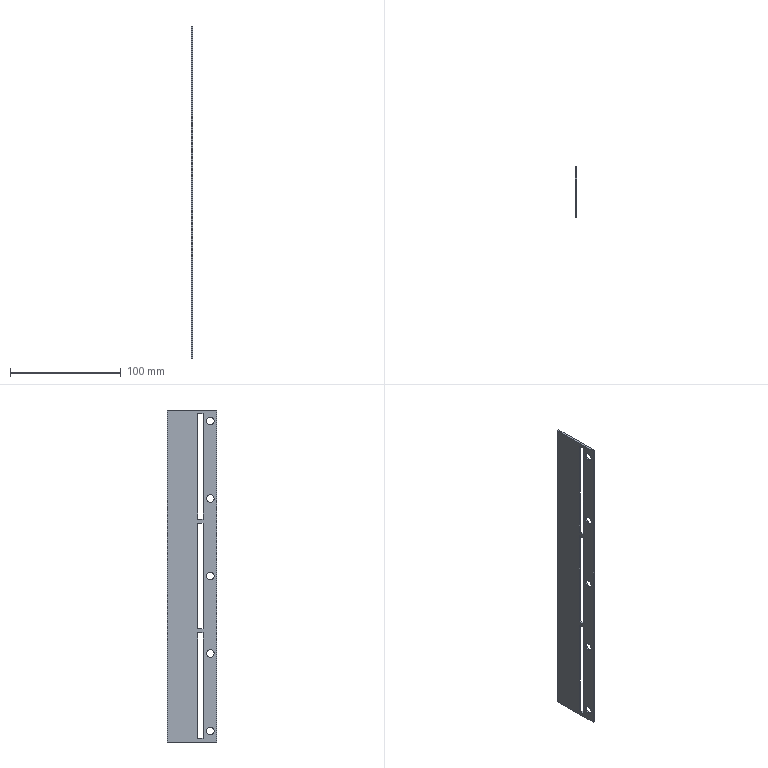Part | STEP file | SYL_0392D6J1SYL0380DJ10-1103933 | 1 solid | 28 faces | box 1.5 x 45 x 300 mm | volume 17824 mm3 | plane 18 | cylinder 10 | commonest cylinder face diameters 7 x10
STEP:
#1=CARTESIAN_POINT('',(0.,6.,-143.5));
#2=VERTEX_POINT('',#1);
#3=CARTESIAN_POINT('',(0.,6.,-136.5));
#4=VERTEX_POINT('',#3);
#5=CARTESIAN_POINT('',(0.,6.,-140.));
#6=DIRECTION('',(1.,0.,0.));
#7=DIRECTION('',(0.,0.,-1.));
#8=AXIS2_PLACEMENT_3D('',#5,#6,#7);
#9=CIRCLE('',#8,3.5);
#10=EDGE_CURVE('',#2,#4,#9,.T.);
#11=ORIENTED_EDGE('',*,*,#10,.F.);
#12=CARTESIAN_POINT('',(1.5,6.,-143.5));
#13=VERTEX_POINT('',#12);
#14=CARTESIAN_POINT('',(1.5,6.,-143.5));
#15=DIRECTION('',(-1.,0.,0.));
#16=VECTOR('',#15,1000.);
#17=LINE('',#14,#16);
#18=EDGE_CURVE('',#13,#2,#17,.T.);
#19=ORIENTED_EDGE('',*,*,#18,.F.);
#20=CARTESIAN_POINT('',(1.5,6.,-136.5));
#21=VERTEX_POINT('',#20);
#22=CARTESIAN_POINT('',(1.5,6.,-140.));
#23=DIRECTION('',(-1.,0.,0.));
#24=DIRECTION('',(0.,0.,1.));
#25=AXIS2_PLACEMENT_3D('',#22,#23,#24);
#26=CIRCLE('',#25,3.5);
#27=EDGE_CURVE('',#21,#13,#26,.T.);
#28=ORIENTED_EDGE('',*,*,#27,.F.);
#29=CARTESIAN_POINT('',(1.5,6.,-136.5));
#30=DIRECTION('',(-1.,0.,0.));
#31=VECTOR('',#30,1000.);
#32=LINE('',#29,#31);
#33=EDGE_CURVE('',#21,#4,#32,.T.);
#34=ORIENTED_EDGE('',*,*,#33,.T.);
#35=EDGE_LOOP('',(#11,#19,#28,#34));
#36=FACE_OUTER_BOUND('',#35,.T.);
#37=CARTESIAN_POINT('',(0.75,6.,-140.));
#38=DIRECTION('',(1.,0.,0.));
#39=DIRECTION('',(0.,0.,-1.));
#40=AXIS2_PLACEMENT_3D('',#37,#38,#39);
#41=CYLINDRICAL_SURFACE('',#40,3.5);
#42=ADVANCED_FACE('',(#36),#41,.F.);
#43=ORIENTED_EDGE('',*,*,#33,.F.);
#44=CARTESIAN_POINT('',(1.5,6.,-140.));
#45=DIRECTION('',(-1.,0.,0.));
#46=DIRECTION('',(0.,0.,-1.));
#47=AXIS2_PLACEMENT_3D('',#44,#45,#46);
#48=CIRCLE('',#47,3.5);
#49=EDGE_CURVE('',#13,#21,#48,.T.);
#50=ORIENTED_EDGE('',*,*,#49,.F.);
#51=ORIENTED_EDGE('',*,*,#18,.T.);
#52=CARTESIAN_POINT('',(0.,6.,-140.));
#53=DIRECTION('',(1.,0.,0.));
#54=DIRECTION('',(0.,0.,1.));
#55=AXIS2_PLACEMENT_3D('',#52,#53,#54);
#56=CIRCLE('',#55,3.5);
#57=EDGE_CURVE('',#4,#2,#56,.T.);
#58=ORIENTED_EDGE('',*,*,#57,.F.);
#59=EDGE_LOOP('',(#43,#50,#51,#58));
#60=FACE_OUTER_BOUND('',#59,.T.);
#61=CARTESIAN_POINT('',(0.75,6.,-140.));
#62=DIRECTION('',(1.,0.,0.));
#63=DIRECTION('',(0.,0.,-1.));
#64=AXIS2_PLACEMENT_3D('',#61,#62,#63);
#65=CYLINDRICAL_SURFACE('',#64,3.5);
#66=ADVANCED_FACE('',(#60),#65,.F.);
#67=CARTESIAN_POINT('',(0.,6.,136.5));
#68=VERTEX_POINT('',#67);
#69=CARTESIAN_POINT('',(0.,6.,143.5));
#70=VERTEX_POINT('',#69);
#71=CARTESIAN_POINT('',(0.,6.,140.));
#72=DIRECTION('',(1.,0.,0.));
#73=DIRECTION('',(0.,0.,-1.));
#74=AXIS2_PLACEMENT_3D('',#71,#72,#73);
#75=CIRCLE('',#74,3.5);
#76=EDGE_CURVE('',#68,#70,#75,.T.);
#77=ORIENTED_EDGE('',*,*,#76,.F.);
#78=CARTESIAN_POINT('',(1.5,6.,136.5));
#79=VERTEX_POINT('',#78);
#80=CARTESIAN_POINT('',(1.5,6.,136.5));
#81=DIRECTION('',(-1.,0.,0.));
#82=VECTOR('',#81,1000.);
#83=LINE('',#80,#82);
#84=EDGE_CURVE('',#79,#68,#83,.T.);
#85=ORIENTED_EDGE('',*,*,#84,.F.);
#86=CARTESIAN_POINT('',(1.5,6.,143.5));
#87=VERTEX_POINT('',#86);
#88=CARTESIAN_POINT('',(1.5,6.,140.));
#89=DIRECTION('',(-1.,0.,0.));
#90=DIRECTION('',(0.,0.,1.));
#91=AXIS2_PLACEMENT_3D('',#88,#89,#90);
#92=CIRCLE('',#91,3.5);
#93=EDGE_CURVE('',#87,#79,#92,.T.);
#94=ORIENTED_EDGE('',*,*,#93,.F.);
#95=CARTESIAN_POINT('',(1.5,6.,143.5));
#96=DIRECTION('',(-1.,0.,0.));
#97=VECTOR('',#96,1000.);
#98=LINE('',#95,#97);
#99=EDGE_CURVE('',#87,#70,#98,.T.);
#100=ORIENTED_EDGE('',*,*,#99,.T.);
#101=EDGE_LOOP('',(#77,#85,#94,#100));
#102=FACE_OUTER_BOUND('',#101,.T.);
#103=CARTESIAN_POINT('',(0.75,6.,140.));
#104=DIRECTION('',(1.,0.,0.));
#105=DIRECTION('',(0.,0.,-1.));
#106=AXIS2_PLACEMENT_3D('',#103,#104,#105);
#107=CYLINDRICAL_SURFACE('',#106,3.5);
#108=ADVANCED_FACE('',(#102),#107,.F.);
#109=ORIENTED_EDGE('',*,*,#99,.F.);
#110=CARTESIAN_POINT('',(1.5,6.,140.));
#111=DIRECTION('',(-1.,0.,0.));
#112=DIRECTION('',(0.,0.,-1.));
#113=AXIS2_PLACEMENT_3D('',#110,#111,#112);
#114=CIRCLE('',#113,3.5);
#115=EDGE_CURVE('',#79,#87,#114,.T.);
#116=ORIENTED_EDGE('',*,*,#115,.F.);
#117=ORIENTED_EDGE('',*,*,#84,.T.);
#118=CARTESIAN_POINT('',(0.,6.,140.));
#119=DIRECTION('',(1.,0.,0.));
#120=DIRECTION('',(0.,0.,1.));
#121=AXIS2_PLACEMENT_3D('',#118,#119,#120);
#122=CIRCLE('',#121,3.5);
#123=EDGE_CURVE('',#70,#68,#122,.T.);
#124=ORIENTED_EDGE('',*,*,#123,.F.);
#125=EDGE_LOOP('',(#109,#116,#117,#124));
#126=FACE_OUTER_BOUND('',#125,.T.);
#127=CARTESIAN_POINT('',(0.75,6.,140.));
#128=DIRECTION('',(1.,0.,0.));
#129=DIRECTION('',(0.,0.,-1.));
#130=AXIS2_PLACEMENT_3D('',#127,#128,#129);
#131=CYLINDRICAL_SURFACE('',#130,3.5);
#132=ADVANCED_FACE('',(#126),#131,.F.);
#133=CARTESIAN_POINT('',(0.,6.,-3.5));
#134=VERTEX_POINT('',#133);
#135=CARTESIAN_POINT('',(0.,6.,3.5));
#136=VERTEX_POINT('',#135);
#137=CARTESIAN_POINT('',(0.,6.,0.));
#138=DIRECTION('',(1.,0.,0.));
#139=DIRECTION('',(0.,0.,-1.));
#140=AXIS2_PLACEMENT_3D('',#137,#138,#139);
#141=CIRCLE('',#140,3.5);
#142=EDGE_CURVE('',#134,#136,#141,.T.);
#143=ORIENTED_EDGE('',*,*,#142,.F.);
#144=CARTESIAN_POINT('',(1.5,6.,-3.5));
#145=VERTEX_POINT('',#144);
#146=CARTESIAN_POINT('',(1.5,6.,-3.5));
#147=DIRECTION('',(-1.,0.,0.));
#148=VECTOR('',#147,1000.);
#149=LINE('',#146,#148);
#150=EDGE_CURVE('',#145,#134,#149,.T.);
#151=ORIENTED_EDGE('',*,*,#150,.F.);
#152=CARTESIAN_POINT('',(1.5,6.,3.5));
#153=VERTEX_POINT('',#152);
#154=CARTESIAN_POINT('',(1.5,6.,0.));
#155=DIRECTION('',(-1.,0.,0.));
#156=DIRECTION('',(0.,0.,1.));
#157=AXIS2_PLACEMENT_3D('',#154,#155,#156);
#158=CIRCLE('',#157,3.5);
#159=EDGE_CURVE('',#153,#145,#158,.T.);
#160=ORIENTED_EDGE('',*,*,#159,.F.);
#161=CARTESIAN_POINT('',(1.5,6.,3.5));
#162=DIRECTION('',(-1.,0.,0.));
#163=VECTOR('',#162,1000.);
#164=LINE('',#161,#163);
#165=EDGE_CURVE('',#153,#136,#164,.T.);
#166=ORIENTED_EDGE('',*,*,#165,.T.);
#167=EDGE_LOOP('',(#143,#151,#160,#166));
#168=FACE_OUTER_BOUND('',#167,.T.);
#169=CARTESIAN_POINT('',(0.75,6.,0.));
#170=DIRECTION('',(1.,0.,0.));
#171=DIRECTION('',(0.,0.,-1.));
#172=AXIS2_PLACEMENT_3D('',#169,#170,#171);
#173=CYLINDRICAL_SURFACE('',#172,3.5);
#174=ADVANCED_FACE('',(#168),#173,.F.);
#175=ORIENTED_EDGE('',*,*,#165,.F.);
#176=CARTESIAN_POINT('',(1.5,6.,0.));
#177=DIRECTION('',(-1.,0.,0.));
#178=DIRECTION('',(0.,0.,-1.));
#179=AXIS2_PLACEMENT_3D('',#176,#177,#178);
#180=CIRCLE('',#179,3.5);
#181=EDGE_CURVE('',#145,#153,#180,.T.);
#182=ORIENTED_EDGE('',*,*,#181,.F.);
#183=ORIENTED_EDGE('',*,*,#150,.T.);
#184=CARTESIAN_POINT('',(0.,6.,0.));
#185=DIRECTION('',(1.,0.,0.));
#186=DIRECTION('',(0.,0.,1.));
#187=AXIS2_PLACEMENT_3D('',#184,#185,#186);
#188=CIRCLE('',#187,3.5);
#189=EDGE_CURVE('',#136,#134,#188,.T.);
#190=ORIENTED_EDGE('',*,*,#189,.F.);
#191=EDGE_LOOP('',(#175,#182,#183,#190));
#192=FACE_OUTER_BOUND('',#191,.T.);
#193=CARTESIAN_POINT('',(0.75,6.,0.));
#194=DIRECTION('',(1.,0.,0.));
#195=DIRECTION('',(0.,0.,-1.));
#196=AXIS2_PLACEMENT_3D('',#193,#194,#195);
#197=CYLINDRICAL_SURFACE('',#196,3.5);
#198=ADVANCED_FACE('',(#192),#197,.F.);
#199=CARTESIAN_POINT('',(0.,6.,-73.5));
#200=VERTEX_POINT('',#199);
#201=CARTESIAN_POINT('',(0.,6.,-66.5));
#202=VERTEX_POINT('',#201);
#203=CARTESIAN_POINT('',(0.,6.,-70.));
#204=DIRECTION('',(1.,0.,0.));
#205=DIRECTION('',(0.,0.,-1.));
#206=AXIS2_PLACEMENT_3D('',#203,#204,#205);
#207=CIRCLE('',#206,3.5);
#208=EDGE_CURVE('',#200,#202,#207,.T.);
#209=ORIENTED_EDGE('',*,*,#208,.F.);
#210=CARTESIAN_POINT('',(1.5,6.,-73.5));
#211=VERTEX_POINT('',#210);
#212=CARTESIAN_POINT('',(1.5,6.,-73.5));
#213=DIRECTION('',(-1.,0.,0.));
#214=VECTOR('',#213,1000.);
#215=LINE('',#212,#214);
#216=EDGE_CURVE('',#211,#200,#215,.T.);
#217=ORIENTED_EDGE('',*,*,#216,.F.);
#218=CARTESIAN_POINT('',(1.5,6.,-66.5));
#219=VERTEX_POINT('',#218);
#220=CARTESIAN_POINT('',(1.5,6.,-70.));
#221=DIRECTION('',(-1.,0.,0.));
#222=DIRECTION('',(0.,0.,1.));
#223=AXIS2_PLACEMENT_3D('',#220,#221,#222);
#224=CIRCLE('',#223,3.5);
#225=EDGE_CURVE('',#219,#211,#224,.T.);
#226=ORIENTED_EDGE('',*,*,#225,.F.);
#227=CARTESIAN_POINT('',(1.5,6.,-66.5));
#228=DIRECTION('',(-1.,0.,0.));
#229=VECTOR('',#228,1000.);
#230=LINE('',#227,#229);
#231=EDGE_CURVE('',#219,#202,#230,.T.);
#232=ORIENTED_EDGE('',*,*,#231,.T.);
#233=EDGE_LOOP('',(#209,#217,#226,#232));
#234=FACE_OUTER_BOUND('',#233,.T.);
#235=CARTESIAN_POINT('',(0.75,6.,-70.));
#236=DIRECTION('',(1.,0.,0.));
#237=DIRECTION('',(0.,0.,-1.));
#238=AXIS2_PLACEMENT_3D('',#235,#236,#237);
#239=CYLINDRICAL_SURFACE('',#238,3.5);
#240=ADVANCED_FACE('',(#234),#239,.F.);
#241=ORIENTED_EDGE('',*,*,#231,.F.);
#242=CARTESIAN_POINT('',(1.5,6.,-70.));
#243=DIRECTION('',(-1.,0.,0.));
#244=DIRECTION('',(0.,0.,-1.));
#245=AXIS2_PLACEMENT_3D('',#242,#243,#244);
#246=CIRCLE('',#245,3.5);
#247=EDGE_CURVE('',#211,#219,#246,.T.);
#248=ORIENTED_EDGE('',*,*,#247,.F.);
#249=ORIENTED_EDGE('',*,*,#216,.T.);
#250=CARTESIAN_POINT('',(0.,6.,-70.));
#251=DIRECTION('',(1.,0.,0.));
#252=DIRECTION('',(0.,0.,1.));
#253=AXIS2_PLACEMENT_3D('',#250,#251,#252);
#254=CIRCLE('',#253,3.5);
#255=EDGE_CURVE('',#202,#200,#254,.T.);
#256=ORIENTED_EDGE('',*,*,#255,.F.);
#257=EDGE_LOOP('',(#241,#248,#249,#256));
#258=FACE_OUTER_BOUND('',#257,.T.);
#259=CARTESIAN_POINT('',(0.75,6.,-70.));
#260=DIRECTION('',(1.,0.,0.));
#261=DIRECTION('',(0.,0.,-1.));
#262=AXIS2_PLACEMENT_3D('',#259,#260,#261);
#263=CYLINDRICAL_SURFACE('',#262,3.5);
#264=ADVANCED_FACE('',(#258),#263,.F.);
#265=CARTESIAN_POINT('',(0.,6.,66.5));
#266=VERTEX_POINT('',#265);
#267=CARTESIAN_POINT('',(0.,6.,73.5));
#268=VERTEX_POINT('',#267);
#269=CARTESIAN_POINT('',(0.,6.,70.));
#270=DIRECTION('',(1.,0.,0.));
#271=DIRECTION('',(0.,0.,-1.));
#272=AXIS2_PLACEMENT_3D('',#269,#270,#271);
#273=CIRCLE('',#272,3.5);
#274=EDGE_CURVE('',#266,#268,#273,.T.);
#275=ORIENTED_EDGE('',*,*,#274,.F.);
#276=CARTESIAN_POINT('',(1.5,6.,66.5));
#277=VERTEX_POINT('',#276);
#278=CARTESIAN_POINT('',(1.5,6.,66.5));
#279=DIRECTION('',(-1.,0.,0.));
#280=VECTOR('',#279,1000.);
#281=LINE('',#278,#280);
#282=EDGE_CURVE('',#277,#266,#281,.T.);
#283=ORIENTED_EDGE('',*,*,#282,.F.);
#284=CARTESIAN_POINT('',(1.5,6.,73.5));
#285=VERTEX_POINT('',#284);
#286=CARTESIAN_POINT('',(1.5,6.,70.));
#287=DIRECTION('',(-1.,0.,0.));
#288=DIRECTION('',(0.,0.,1.));
#289=AXIS2_PLACEMENT_3D('',#286,#287,#288);
#290=CIRCLE('',#289,3.5);
#291=EDGE_CURVE('',#285,#277,#290,.T.);
#292=ORIENTED_EDGE('',*,*,#291,.F.);
#293=CARTESIAN_POINT('',(1.5,6.,73.5));
#294=DIRECTION('',(-1.,0.,0.));
#295=VECTOR('',#294,1000.);
#296=LINE('',#293,#295);
#297=EDGE_CURVE('',#285,#268,#296,.T.);
#298=ORIENTED_EDGE('',*,*,#297,.T.);
#299=EDGE_LOOP('',(#275,#283,#292,#298));
#300=FACE_OUTER_BOUND('',#299,.T.);
#301=CARTESIAN_POINT('',(0.75,6.,70.));
#302=DIRECTION('',(1.,0.,0.));
#303=DIRECTION('',(0.,0.,-1.));
#304=AXIS2_PLACEMENT_3D('',#301,#302,#303);
#305=CYLINDRICAL_SURFACE('',#304,3.5);
#306=ADVANCED_FACE('',(#300),#305,.F.);
#307=ORIENTED_EDGE('',*,*,#297,.F.);
#308=CARTESIAN_POINT('',(1.5,6.,70.));
#309=DIRECTION('',(-1.,0.,0.));
#310=DIRECTION('',(0.,0.,-1.));
#311=AXIS2_PLACEMENT_3D('',#308,#309,#310);
#312=CIRCLE('',#311,3.5);
#313=EDGE_CURVE('',#277,#285,#312,.T.);
#314=ORIENTED_EDGE('',*,*,#313,.F.);
#315=ORIENTED_EDGE('',*,*,#282,.T.);
#316=CARTESIAN_POINT('',(0.,6.,70.));
#317=DIRECTION('',(1.,0.,0.));
#318=DIRECTION('',(0.,0.,1.));
#319=AXIS2_PLACEMENT_3D('',#316,#317,#318);
#320=CIRCLE('',#319,3.5);
#321=EDGE_CURVE('',#268,#266,#320,.T.);
#322=ORIENTED_EDGE('',*,*,#321,.F.);
#323=EDGE_LOOP('',(#307,#314,#315,#322));
#324=FACE_OUTER_BOUND('',#323,.T.);
#325=CARTESIAN_POINT('',(0.75,6.,70.));
#326=DIRECTION('',(1.,0.,0.));
#327=DIRECTION('',(0.,0.,-1.));
#328=AXIS2_PLACEMENT_3D('',#325,#326,#327);
#329=CYLINDRICAL_SURFACE('',#328,3.5);
#330=ADVANCED_FACE('',(#324),#329,.F.);
#331=CARTESIAN_POINT('',(1.5,17.5,-47.5));
#332=VERTEX_POINT('',#331);
#333=CARTESIAN_POINT('',(0.,17.5,-47.5));
#334=VERTEX_POINT('',#333);
#335=CARTESIAN_POINT('',(1.5,17.5,-47.5));
#336=DIRECTION('',(-1.,0.,0.));
#337=VECTOR('',#336,1000.);
#338=LINE('',#335,#337);
#339=EDGE_CURVE('',#332,#334,#338,.T.);
#340=ORIENTED_EDGE('',*,*,#339,.T.);
#341=CARTESIAN_POINT('',(0.,12.5,-47.5));
#342=VERTEX_POINT('',#341);
#343=CARTESIAN_POINT('',(0.,12.5,-47.5));
#344=DIRECTION('',(0.,1.,0.));
#345=VECTOR('',#344,1000.);
#346=LINE('',#343,#345);
#347=EDGE_CURVE('',#342,#334,#346,.T.);
#348=ORIENTED_EDGE('',*,*,#347,.F.);
#349=CARTESIAN_POINT('',(1.5,12.5,-47.5));
#350=VERTEX_POINT('',#349);
#351=CARTESIAN_POINT('',(1.5,12.5,-47.5));
#352=DIRECTION('',(-1.,0.,0.));
#353=VECTOR('',#352,1000.);
#354=LINE('',#351,#353);
#355=EDGE_CURVE('',#350,#342,#354,.T.);
#356=ORIENTED_EDGE('',*,*,#355,.F.);
#357=CARTESIAN_POINT('',(1.5,12.5,-47.5));
#358=DIRECTION('',(0.,1.,0.));
#359=VECTOR('',#358,1000.);
#360=LINE('',#357,#359);
#361=EDGE_CURVE('',#350,#332,#360,.T.);
#362=ORIENTED_EDGE('',*,*,#361,.T.);
#363=EDGE_LOOP('',(#340,#348,#356,#362));
#364=FACE_OUTER_BOUND('',#363,.T.);
#365=CARTESIAN_POINT('',(0.75,15.,-47.5));
#366=DIRECTION('',(0.,0.,-1.));
#367=DIRECTION('',(0.,-1.,0.));
#368=AXIS2_PLACEMENT_3D('',#365,#366,#367);
#369=PLANE('',#368);
#370=ADVANCED_FACE('',(#364),#369,.F.);
#371=CARTESIAN_POINT('',(0.,17.5,47.5));
#372=VERTEX_POINT('',#371);
#373=CARTESIAN_POINT('',(1.5,17.5,47.5));
#374=VERTEX_POINT('',#373);
#375=CARTESIAN_POINT('',(0.,17.5,47.5));
#376=DIRECTION('',(1.,0.,0.));
#377=VECTOR('',#376,1000.);
#378=LINE('',#375,#377);
#379=EDGE_CURVE('',#372,#374,#378,.T.);
#380=ORIENTED_EDGE('',*,*,#379,.F.);
#381=CARTESIAN_POINT('',(0.,17.5,-47.5));
#382=DIRECTION('',(0.,0.,1.));
#383=VECTOR('',#382,1000.);
#384=LINE('',#381,#383);
#385=EDGE_CURVE('',#334,#372,#384,.T.);
#386=ORIENTED_EDGE('',*,*,#385,.F.);
#387=ORIENTED_EDGE('',*,*,#339,.F.);
#388=CARTESIAN_POINT('',(1.5,17.5,-47.5));
#389=DIRECTION('',(0.,0.,1.));
#390=VECTOR('',#389,1000.);
#391=LINE('',#388,#390);
#392=EDGE_CURVE('',#332,#374,#391,.T.);
#393=ORIENTED_EDGE('',*,*,#392,.T.);
#394=EDGE_LOOP('',(#380,#386,#387,#393));
#395=FACE_OUTER_BOUND('',#394,.T.);
#396=CARTESIAN_POINT('',(0.75,17.5,0.));
#397=DIRECTION('',(0.,1.,0.));
#398=DIRECTION('',(1.,0.,0.));
#399=AXIS2_PLACEMENT_3D('',#396,#397,#398);
#400=PLANE('',#399);
#401=ADVANCED_FACE('',(#395),#400,.F.);
#402=CARTESIAN_POINT('',(1.5,12.5,47.5));
#403=VERTEX_POINT('',#402);
#404=CARTESIAN_POINT('',(0.,12.5,47.5));
#405=VERTEX_POINT('',#404);
#406=CARTESIAN_POINT('',(1.5,12.5,47.5));
#407=DIRECTION('',(-1.,0.,0.));
#408=VECTOR('',#407,1000.);
#409=LINE('',#406,#408);
#410=EDGE_CURVE('',#403,#405,#409,.T.);
#411=ORIENTED_EDGE('',*,*,#410,.T.);
#412=CARTESIAN_POINT('',(0.,17.5,47.5));
#413=DIRECTION('',(0.,-1.,0.));
#414=VECTOR('',#413,1000.);
#415=LINE('',#412,#414);
#416=EDGE_CURVE('',#372,#405,#415,.T.);
#417=ORIENTED_EDGE('',*,*,#416,.F.);
#418=ORIENTED_EDGE('',*,*,#379,.T.);
#419=CARTESIAN_POINT('',(1.5,17.5,47.5));
#420=DIRECTION('',(0.,-1.,0.));
#421=VECTOR('',#420,1000.);
#422=LINE('',#419,#421);
#423=EDGE_CURVE('',#374,#403,#422,.T.);
#424=ORIENTED_EDGE('',*,*,#423,.T.);
#425=EDGE_LOOP('',(#411,#417,#418,#424));
#426=FACE_OUTER_BOUND('',#425,.T.);
#427=CARTESIAN_POINT('',(0.75,15.,47.5));
#428=DIRECTION('',(0.,0.,1.));
#429=DIRECTION('',(1.,0.,0.));
#430=AXIS2_PLACEMENT_3D('',#427,#428,#429);
#431=PLANE('',#430);
#432=ADVANCED_FACE('',(#426),#431,.F.);
#433=CARTESIAN_POINT('',(1.5,17.5,-146.5));
#434=VERTEX_POINT('',#433);
#435=CARTESIAN_POINT('',(0.,17.5,-146.5));
#436=VERTEX_POINT('',#435);
#437=CARTESIAN_POINT('',(1.5,17.5,-146.5));
#438=DIRECTION('',(-1.,0.,0.));
#439=VECTOR('',#438,1000.);
#440=LINE('',#437,#439);
#441=EDGE_CURVE('',#434,#436,#440,.T.);
#442=ORIENTED_EDGE('',*,*,#441,.T.);
#443=CARTESIAN_POINT('',(0.,12.5,-146.5));
#444=VERTEX_POINT('',#443);
#445=CARTESIAN_POINT('',(0.,12.5,-146.5));
#446=DIRECTION('',(0.,1.,0.));
#447=VECTOR('',#446,1000.);
#448=LINE('',#445,#447);
#449=EDGE_CURVE('',#444,#436,#448,.T.);
#450=ORIENTED_EDGE('',*,*,#449,.F.);
#451=CARTESIAN_POINT('',(1.5,12.5,-146.5));
#452=VERTEX_POINT('',#451);
#453=CARTESIAN_POINT('',(1.5,12.5,-146.5));
#454=DIRECTION('',(-1.,0.,0.));
#455=VECTOR('',#454,1000.);
#456=LINE('',#453,#455);
#457=EDGE_CURVE('',#452,#444,#456,.T.);
#458=ORIENTED_EDGE('',*,*,#457,.F.);
#459=CARTESIAN_POINT('',(1.5,12.5,-146.5));
#460=DIRECTION('',(0.,1.,0.));
#461=VECTOR('',#460,1000.);
#462=LINE('',#459,#461);
#463=EDGE_CURVE('',#452,#434,#462,.T.);
#464=ORIENTED_EDGE('',*,*,#463,.T.);
#465=EDGE_LOOP('',(#442,#450,#458,#464));
#466=FACE_OUTER_BOUND('',#465,.T.);
#467=CARTESIAN_POINT('',(0.75,15.,-146.5));
#468=DIRECTION('',(0.,0.,-1.));
#469=DIRECTION('',(0.,-1.,0.));
#470=AXIS2_PLACEMENT_3D('',#467,#468,#469);
#471=PLANE('',#470);
#472=ADVANCED_FACE('',(#466),#471,.F.);
#473=CARTESIAN_POINT('',(0.,17.5,-51.5));
#474=VERTEX_POINT('',#473);
#475=CARTESIAN_POINT('',(1.5,17.5,-51.5));
#476=VERTEX_POINT('',#475);
#477=CARTESIAN_POINT('',(0.,17.5,-51.5));
#478=DIRECTION('',(1.,0.,0.));
#479=VECTOR('',#478,1000.);
#480=LINE('',#477,#479);
#481=EDGE_CURVE('',#474,#476,#480,.T.);
#482=ORIENTED_EDGE('',*,*,#481,.F.);
#483=CARTESIAN_POINT('',(0.,17.5,-146.5));
#484=DIRECTION('',(0.,0.,1.));
#485=VECTOR('',#484,1000.);
#486=LINE('',#483,#485);
#487=EDGE_CURVE('',#436,#474,#486,.T.);
#488=ORIENTED_EDGE('',*,*,#487,.F.);
#489=ORIENTED_EDGE('',*,*,#441,.F.);
#490=CARTESIAN_POINT('',(1.5,17.5,-146.5));
#491=DIRECTION('',(0.,0.,1.));
#492=VECTOR('',#491,1000.);
#493=LINE('',#490,#492);
#494=EDGE_CURVE('',#434,#476,#493,.T.);
#495=ORIENTED_EDGE('',*,*,#494,.T.);
#496=EDGE_LOOP('',(#482,#488,#489,#495));
#497=FACE_OUTER_BOUND('',#496,.T.);
#498=CARTESIAN_POINT('',(0.75,17.5,-99.));
#499=DIRECTION('',(0.,1.,0.));
#500=DIRECTION('',(1.,0.,0.));
#501=AXIS2_PLACEMENT_3D('',#498,#499,#500);
#502=PLANE('',#501);
#503=ADVANCED_FACE('',(#497),#502,.F.);
#504=CARTESIAN_POINT('',(1.5,12.5,-51.5));
#505=VERTEX_POINT('',#504);
#506=CARTESIAN_POINT('',(0.,12.5,-51.5));
#507=VERTEX_POINT('',#506);
#508=CARTESIAN_POINT('',(1.5,12.5,-51.5));
#509=DIRECTION('',(-1.,0.,0.));
#510=VECTOR('',#509,1000.);
#511=LINE('',#508,#510);
#512=EDGE_CURVE('',#505,#507,#511,.T.);
#513=ORIENTED_EDGE('',*,*,#512,.T.);
#514=CARTESIAN_POINT('',(0.,17.5,-51.5));
#515=DIRECTION('',(0.,-1.,0.));
#516=VECTOR('',#515,1000.);
#517=LINE('',#514,#516);
#518=EDGE_CURVE('',#474,#507,#517,.T.);
#519=ORIENTED_EDGE('',*,*,#518,.F.);
#520=ORIENTED_EDGE('',*,*,#481,.T.);
#521=CARTESIAN_POINT('',(1.5,17.5,-51.5));
#522=DIRECTION('',(0.,-1.,0.));
#523=VECTOR('',#522,1000.);
#524=LINE('',#521,#523);
#525=EDGE_CURVE('',#476,#505,#524,.T.);
#526=ORIENTED_EDGE('',*,*,#525,.T.);
#527=EDGE_LOOP('',(#513,#519,#520,#526));
#528=FACE_OUTER_BOUND('',#527,.T.);
#529=CARTESIAN_POINT('',(0.75,15.,-51.5));
#530=DIRECTION('',(0.,0.,1.));
#531=DIRECTION('',(1.,0.,0.));
#532=AXIS2_PLACEMENT_3D('',#529,#530,#531);
#533=PLANE('',#532);
#534=ADVANCED_FACE('',(#528),#533,.F.);
#535=ORIENTED_EDGE('',*,*,#457,.T.);
#536=CARTESIAN_POINT('',(0.,12.5,-51.5));
#537=DIRECTION('',(0.,0.,-1.));
#538=VECTOR('',#537,1000.);
#539=LINE('',#536,#538);
#540=EDGE_CURVE('',#507,#444,#539,.T.);
#541=ORIENTED_EDGE('',*,*,#540,.F.);
#542=ORIENTED_EDGE('',*,*,#512,.F.);
#543=CARTESIAN_POINT('',(1.5,12.5,-51.5));
#544=DIRECTION('',(0.,0.,-1.));
#545=VECTOR('',#544,1000.);
#546=LINE('',#543,#545);
#547=EDGE_CURVE('',#505,#452,#546,.T.);
#548=ORIENTED_EDGE('',*,*,#547,.T.);
#549=EDGE_LOOP('',(#535,#541,#542,#548));
#550=FACE_OUTER_BOUND('',#549,.T.);
#551=CARTESIAN_POINT('',(0.75,12.5,-99.));
#552=DIRECTION('',(0.,-1.,0.));
#553=DIRECTION('',(0.,0.,-1.));
#554=AXIS2_PLACEMENT_3D('',#551,#552,#553);
#555=PLANE('',#554);
#556=ADVANCED_FACE('',(#550),#555,.F.);
#557=CARTESIAN_POINT('',(1.5,17.5,51.5));
#558=VERTEX_POINT('',#557);
#559=CARTESIAN_POINT('',(0.,17.5,51.5));
#560=VERTEX_POINT('',#559);
#561=CARTESIAN_POINT('',(1.5,17.5,51.5));
#562=DIRECTION('',(-1.,0.,0.));
#563=VECTOR('',#562,1000.);
#564=LINE('',#561,#563);
#565=EDGE_CURVE('',#558,#560,#564,.T.);
#566=ORIENTED_EDGE('',*,*,#565,.T.);
#567=CARTESIAN_POINT('',(0.,12.5,51.5));
#568=VERTEX_POINT('',#567);
#569=CARTESIAN_POINT('',(0.,12.5,51.5));
#570=DIRECTION('',(0.,1.,0.));
#571=VECTOR('',#570,1000.);
#572=LINE('',#569,#571);
#573=EDGE_CURVE('',#568,#560,#572,.T.);
#574=ORIENTED_EDGE('',*,*,#573,.F.);
#575=CARTESIAN_POINT('',(1.5,12.5,51.5));
#576=VERTEX_POINT('',#575);
#577=CARTESIAN_POINT('',(1.5,12.5,51.5));
#578=DIRECTION('',(-1.,0.,0.));
#579=VECTOR('',#578,1000.);
#580=LINE('',#577,#579);
#581=EDGE_CURVE('',#576,#568,#580,.T.);
#582=ORIENTED_EDGE('',*,*,#581,.F.);
#583=CARTESIAN_POINT('',(1.5,12.5,51.5));
#584=DIRECTION('',(0.,1.,0.));
#585=VECTOR('',#584,1000.);
#586=LINE('',#583,#585);
#587=EDGE_CURVE('',#576,#558,#586,.T.);
#588=ORIENTED_EDGE('',*,*,#587,.T.);
#589=EDGE_LOOP('',(#566,#574,#582,#588));
#590=FACE_OUTER_BOUND('',#589,.T.);
#591=CARTESIAN_POINT('',(0.75,15.,51.5));
#592=DIRECTION('',(0.,0.,-1.));
#593=DIRECTION('',(0.,-1.,0.));
#594=AXIS2_PLACEMENT_3D('',#591,#592,#593);
#595=PLANE('',#594);
#596=ADVANCED_FACE('',(#590),#595,.F.);
#597=CARTESIAN_POINT('',(0.,17.5,146.5));
#598=VERTEX_POINT('',#597);
#599=CARTESIAN_POINT('',(1.5,17.5,146.5));
#600=VERTEX_POINT('',#599);
#601=CARTESIAN_POINT('',(0.,17.5,146.5));
#602=DIRECTION('',(1.,0.,0.));
#603=VECTOR('',#602,1000.);
#604=LINE('',#601,#603);
#605=EDGE_CURVE('',#598,#600,#604,.T.);
#606=ORIENTED_EDGE('',*,*,#605,.F.);
#607=CARTESIAN_POINT('',(0.,17.5,51.5));
#608=DIRECTION('',(0.,0.,1.));
#609=VECTOR('',#608,1000.);
#610=LINE('',#607,#609);
#611=EDGE_CURVE('',#560,#598,#610,.T.);
#612=ORIENTED_EDGE('',*,*,#611,.F.);
#613=ORIENTED_EDGE('',*,*,#565,.F.);
#614=CARTESIAN_POINT('',(1.5,17.5,51.5));
#615=DIRECTION('',(0.,0.,1.));
#616=VECTOR('',#615,1000.);
#617=LINE('',#614,#616);
#618=EDGE_CURVE('',#558,#600,#617,.T.);
#619=ORIENTED_EDGE('',*,*,#618,.T.);
#620=EDGE_LOOP('',(#606,#612,#613,#619));
#621=FACE_OUTER_BOUND('',#620,.T.);
#622=CARTESIAN_POINT('',(0.75,17.5,99.));
#623=DIRECTION('',(0.,1.,0.));
#624=DIRECTION('',(1.,0.,0.));
#625=AXIS2_PLACEMENT_3D('',#622,#623,#624);
#626=PLANE('',#625);
#627=ADVANCED_FACE('',(#621),#626,.F.);
#628=CARTESIAN_POINT('',(1.5,12.5,146.5));
#629=VERTEX_POINT('',#628);
#630=CARTESIAN_POINT('',(0.,12.5,146.5));
#631=VERTEX_POINT('',#630);
#632=CARTESIAN_POINT('',(1.5,12.5,146.5));
#633=DIRECTION('',(-1.,0.,0.));
#634=VECTOR('',#633,1000.);
#635=LINE('',#632,#634);
#636=EDGE_CURVE('',#629,#631,#635,.T.);
#637=ORIENTED_EDGE('',*,*,#636,.T.);
#638=CARTESIAN_POINT('',(0.,17.5,146.5));
#639=DIRECTION('',(0.,-1.,0.));
#640=VECTOR('',#639,1000.);
#641=LINE('',#638,#640);
#642=EDGE_CURVE('',#598,#631,#641,.T.);
#643=ORIENTED_EDGE('',*,*,#642,.F.);
#644=ORIENTED_EDGE('',*,*,#605,.T.);
#645=CARTESIAN_POINT('',(1.5,17.5,146.5));
#646=DIRECTION('',(0.,-1.,0.));
#647=VECTOR('',#646,1000.);
#648=LINE('',#645,#647);
#649=EDGE_CURVE('',#600,#629,#648,.T.);
#650=ORIENTED_EDGE('',*,*,#649,.T.);
#651=EDGE_LOOP('',(#637,#643,#644,#650));
#652=FACE_OUTER_BOUND('',#651,.T.);
#653=CARTESIAN_POINT('',(0.75,15.,146.5));
#654=DIRECTION('',(0.,0.,1.));
#655=DIRECTION('',(1.,0.,0.));
#656=AXIS2_PLACEMENT_3D('',#653,#654,#655);
#657=PLANE('',#656);
#658=ADVANCED_FACE('',(#652),#657,.F.);
#659=ORIENTED_EDGE('',*,*,#581,.T.);
#660=CARTESIAN_POINT('',(0.,12.5,146.5));
#661=DIRECTION('',(0.,0.,-1.));
#662=VECTOR('',#661,1000.);
#663=LINE('',#660,#662);
#664=EDGE_CURVE('',#631,#568,#663,.T.);
#665=ORIENTED_EDGE('',*,*,#664,.F.);
#666=ORIENTED_EDGE('',*,*,#636,.F.);
#667=CARTESIAN_POINT('',(1.5,12.5,146.5));
#668=DIRECTION('',(0.,0.,-1.));
#669=VECTOR('',#668,1000.);
#670=LINE('',#667,#669);
#671=EDGE_CURVE('',#629,#576,#670,.T.);
#672=ORIENTED_EDGE('',*,*,#671,.T.);
#673=EDGE_LOOP('',(#659,#665,#666,#672));
#674=FACE_OUTER_BOUND('',#673,.T.);
#675=CARTESIAN_POINT('',(0.75,12.5,99.));
#676=DIRECTION('',(0.,-1.,0.));
#677=DIRECTION('',(0.,0.,-1.));
#678=AXIS2_PLACEMENT_3D('',#675,#676,#677);
#679=PLANE('',#678);
#680=ADVANCED_FACE('',(#674),#679,.F.);
#681=ORIENTED_EDGE('',*,*,#10,.T.);
#682=ORIENTED_EDGE('',*,*,#57,.T.);
#683=EDGE_LOOP('',(#681,#682));
#684=FACE_BOUND('',#683,.T.);
#685=ORIENTED_EDGE('',*,*,#76,.T.);
#686=ORIENTED_EDGE('',*,*,#123,.T.);
#687=EDGE_LOOP('',(#685,#686));
#688=FACE_BOUND('',#687,.T.);
#689=ORIENTED_EDGE('',*,*,#142,.T.);
#690=ORIENTED_EDGE('',*,*,#189,.T.);
#691=EDGE_LOOP('',(#689,#690));
#692=FACE_BOUND('',#691,.T.);
#693=ORIENTED_EDGE('',*,*,#208,.T.);
#694=ORIENTED_EDGE('',*,*,#255,.T.);
#695=EDGE_LOOP('',(#693,#694));
#696=FACE_BOUND('',#695,.T.);
#697=ORIENTED_EDGE('',*,*,#274,.T.);
#698=ORIENTED_EDGE('',*,*,#321,.T.);
#699=EDGE_LOOP('',(#697,#698));
#700=FACE_BOUND('',#699,.T.);
#701=ORIENTED_EDGE('',*,*,#347,.T.);
#702=ORIENTED_EDGE('',*,*,#385,.T.);
#703=ORIENTED_EDGE('',*,*,#416,.T.);
#704=CARTESIAN_POINT('',(0.,12.5,47.5));
#705=DIRECTION('',(0.,0.,-1.));
#706=VECTOR('',#705,1000.);
#707=LINE('',#704,#706);
#708=EDGE_CURVE('',#405,#342,#707,.T.);
#709=ORIENTED_EDGE('',*,*,#708,.T.);
#710=EDGE_LOOP('',(#701,#702,#703,#709));
#711=FACE_BOUND('',#710,.T.);
#712=ORIENTED_EDGE('',*,*,#449,.T.);
#713=ORIENTED_EDGE('',*,*,#487,.T.);
#714=ORIENTED_EDGE('',*,*,#518,.T.);
#715=ORIENTED_EDGE('',*,*,#540,.T.);
#716=EDGE_LOOP('',(#712,#713,#714,#715));
#717=FACE_BOUND('',#716,.T.);
#718=ORIENTED_EDGE('',*,*,#573,.T.);
#719=ORIENTED_EDGE('',*,*,#611,.T.);
#720=ORIENTED_EDGE('',*,*,#642,.T.);
#721=ORIENTED_EDGE('',*,*,#664,.T.);
#722=EDGE_LOOP('',(#718,#719,#720,#721));
#723=FACE_BOUND('',#722,.T.);
#724=CARTESIAN_POINT('',(0.,0.,-150.));
#725=VERTEX_POINT('',#724);
#726=CARTESIAN_POINT('',(0.,0.,150.));
#727=VERTEX_POINT('',#726);
#728=CARTESIAN_POINT('',(0.,0.,-150.));
#729=DIRECTION('',(0.,0.,1.));
#730=VECTOR('',#729,1000.);
#731=LINE('',#728,#730);
#732=EDGE_CURVE('',#725,#727,#731,.T.);
#733=ORIENTED_EDGE('',*,*,#732,.T.);
#734=CARTESIAN_POINT('',(0.,45.,150.));
#735=VERTEX_POINT('',#734);
#736=CARTESIAN_POINT('',(0.,0.,150.));
#737=DIRECTION('',(0.,1.,0.));
#738=VECTOR('',#737,1000.);
#739=LINE('',#736,#738);
#740=EDGE_CURVE('',#727,#735,#739,.T.);
#741=ORIENTED_EDGE('',*,*,#740,.T.);
#742=CARTESIAN_POINT('',(0.,45.,-150.));
#743=VERTEX_POINT('',#742);
#744=CARTESIAN_POINT('',(0.,45.,150.));
#745=DIRECTION('',(0.,0.,-1.));
#746=VECTOR('',#745,1000.);
#747=LINE('',#744,#746);
#748=EDGE_CURVE('',#735,#743,#747,.T.);
#749=ORIENTED_EDGE('',*,*,#748,.T.);
#750=CARTESIAN_POINT('',(0.,45.,-150.));
#751=DIRECTION('',(0.,-1.,0.));
#752=VECTOR('',#751,1000.);
#753=LINE('',#750,#752);
#754=EDGE_CURVE('',#743,#725,#753,.T.);
#755=ORIENTED_EDGE('',*,*,#754,.T.);
#756=EDGE_LOOP('',(#733,#741,#749,#755));
#757=FACE_OUTER_BOUND('',#756,.T.);
#758=CARTESIAN_POINT('',(0.,0.,0.));
#759=DIRECTION('',(1.,0.,0.));
#760=DIRECTION('',(0.,1.,0.));
#761=AXIS2_PLACEMENT_3D('',#758,#759,#760);
#762=PLANE('',#761);
#763=ADVANCED_FACE('',(#684,#688,#692,#696,#700,#711,#717,#723,#757),#762,.F.);
#764=CARTESIAN_POINT('',(1.5,0.,-150.));
#765=VERTEX_POINT('',#764);
#766=CARTESIAN_POINT('',(1.5,0.,-150.));
#767=DIRECTION('',(-1.,0.,0.));
#768=VECTOR('',#767,1000.);
#769=LINE('',#766,#768);
#770=EDGE_CURVE('',#765,#725,#769,.T.);
#771=ORIENTED_EDGE('',*,*,#770,.T.);
#772=ORIENTED_EDGE('',*,*,#754,.F.);
#773=CARTESIAN_POINT('',(1.5,45.,-150.));
#774=VERTEX_POINT('',#773);
#775=CARTESIAN_POINT('',(1.5,45.,-150.));
#776=DIRECTION('',(-1.,0.,0.));
#777=VECTOR('',#776,1000.);
#778=LINE('',#775,#777);
#779=EDGE_CURVE('',#774,#743,#778,.T.);
#780=ORIENTED_EDGE('',*,*,#779,.F.);
#781=CARTESIAN_POINT('',(1.5,45.,-150.));
#782=DIRECTION('',(0.,-1.,0.));
#783=VECTOR('',#782,1000.);
#784=LINE('',#781,#783);
#785=EDGE_CURVE('',#774,#765,#784,.T.);
#786=ORIENTED_EDGE('',*,*,#785,.T.);
#787=EDGE_LOOP('',(#771,#772,#780,#786));
#788=FACE_OUTER_BOUND('',#787,.T.);
#789=CARTESIAN_POINT('',(0.75,22.5,-150.));
#790=DIRECTION('',(0.,0.,1.));
#791=DIRECTION('',(1.,0.,0.));
#792=AXIS2_PLACEMENT_3D('',#789,#790,#791);
#793=PLANE('',#792);
#794=ADVANCED_FACE('',(#788),#793,.F.);
#795=CARTESIAN_POINT('',(1.5,0.,150.));
#796=VERTEX_POINT('',#795);
#797=CARTESIAN_POINT('',(1.5,0.,150.));
#798=DIRECTION('',(-1.,0.,0.));
#799=VECTOR('',#798,1000.);
#800=LINE('',#797,#799);
#801=EDGE_CURVE('',#796,#727,#800,.T.);
#802=ORIENTED_EDGE('',*,*,#801,.T.);
#803=ORIENTED_EDGE('',*,*,#732,.F.);
#804=ORIENTED_EDGE('',*,*,#770,.F.);
#805=CARTESIAN_POINT('',(1.5,0.,-150.));
#806=DIRECTION('',(0.,0.,1.));
#807=VECTOR('',#806,1000.);
#808=LINE('',#805,#807);
#809=EDGE_CURVE('',#765,#796,#808,.T.);
#810=ORIENTED_EDGE('',*,*,#809,.T.);
#811=EDGE_LOOP('',(#802,#803,#804,#810));
#812=FACE_OUTER_BOUND('',#811,.T.);
#813=CARTESIAN_POINT('',(0.75,0.,0.));
#814=DIRECTION('',(0.,1.,0.));
#815=DIRECTION('',(1.,0.,0.));
#816=AXIS2_PLACEMENT_3D('',#813,#814,#815);
#817=PLANE('',#816);
#818=ADVANCED_FACE('',(#812),#817,.F.);
#819=CARTESIAN_POINT('',(1.5,45.,150.));
#820=VERTEX_POINT('',#819);
#821=CARTESIAN_POINT('',(0.,45.,150.));
#822=DIRECTION('',(1.,0.,0.));
#823=VECTOR('',#822,1000.);
#824=LINE('',#821,#823);
#825=EDGE_CURVE('',#735,#820,#824,.T.);
#826=ORIENTED_EDGE('',*,*,#825,.F.);
#827=ORIENTED_EDGE('',*,*,#740,.F.);
#828=ORIENTED_EDGE('',*,*,#801,.F.);
#829=CARTESIAN_POINT('',(1.5,0.,150.));
#830=DIRECTION('',(0.,1.,0.));
#831=VECTOR('',#830,1000.);
#832=LINE('',#829,#831);
#833=EDGE_CURVE('',#796,#820,#832,.T.);
#834=ORIENTED_EDGE('',*,*,#833,.T.);
#835=EDGE_LOOP('',(#826,#827,#828,#834));
#836=FACE_OUTER_BOUND('',#835,.T.);
#837=CARTESIAN_POINT('',(0.75,22.5,150.));
#838=DIRECTION('',(0.,0.,-1.));
#839=DIRECTION('',(0.,-1.,0.));
#840=AXIS2_PLACEMENT_3D('',#837,#838,#839);
#841=PLANE('',#840);
#842=ADVANCED_FACE('',(#836),#841,.F.);
#843=ORIENTED_EDGE('',*,*,#779,.T.);
#844=ORIENTED_EDGE('',*,*,#748,.F.);
#845=ORIENTED_EDGE('',*,*,#825,.T.);
#846=CARTESIAN_POINT('',(1.5,45.,150.));
#847=DIRECTION('',(0.,0.,-1.));
#848=VECTOR('',#847,1000.);
#849=LINE('',#846,#848);
#850=EDGE_CURVE('',#820,#774,#849,.T.);
#851=ORIENTED_EDGE('',*,*,#850,.T.);
#852=EDGE_LOOP('',(#843,#844,#845,#851));
#853=FACE_OUTER_BOUND('',#852,.T.);
#854=CARTESIAN_POINT('',(0.75,45.,0.));
#855=DIRECTION('',(0.,-1.,0.));
#856=DIRECTION('',(0.,0.,-1.));
#857=AXIS2_PLACEMENT_3D('',#854,#855,#856);
#858=PLANE('',#857);
#859=ADVANCED_FACE('',(#853),#858,.F.);
#860=ORIENTED_EDGE('',*,*,#291,.T.);
#861=ORIENTED_EDGE('',*,*,#313,.T.);
#862=EDGE_LOOP('',(#860,#861));
#863=FACE_BOUND('',#862,.T.);
#864=ORIENTED_EDGE('',*,*,#225,.T.);
#865=ORIENTED_EDGE('',*,*,#247,.T.);
#866=EDGE_LOOP('',(#864,#865));
#867=FACE_BOUND('',#866,.T.);
#868=ORIENTED_EDGE('',*,*,#159,.T.);
#869=ORIENTED_EDGE('',*,*,#181,.T.);
#870=EDGE_LOOP('',(#868,#869));
#871=FACE_BOUND('',#870,.T.);
#872=ORIENTED_EDGE('',*,*,#93,.T.);
#873=ORIENTED_EDGE('',*,*,#115,.T.);
#874=EDGE_LOOP('',(#872,#873));
#875=FACE_BOUND('',#874,.T.);
#876=ORIENTED_EDGE('',*,*,#27,.T.);
#877=ORIENTED_EDGE('',*,*,#49,.T.);
#878=EDGE_LOOP('',(#876,#877));
#879=FACE_BOUND('',#878,.T.);
#880=ORIENTED_EDGE('',*,*,#392,.F.);
#881=ORIENTED_EDGE('',*,*,#361,.F.);
#882=CARTESIAN_POINT('',(1.5,12.5,47.5));
#883=DIRECTION('',(0.,0.,-1.));
#884=VECTOR('',#883,1000.);
#885=LINE('',#882,#884);
#886=EDGE_CURVE('',#403,#350,#885,.T.);
#887=ORIENTED_EDGE('',*,*,#886,.F.);
#888=ORIENTED_EDGE('',*,*,#423,.F.);
#889=EDGE_LOOP('',(#880,#881,#887,#888));
#890=FACE_BOUND('',#889,.T.);
#891=ORIENTED_EDGE('',*,*,#494,.F.);
#892=ORIENTED_EDGE('',*,*,#463,.F.);
#893=ORIENTED_EDGE('',*,*,#547,.F.);
#894=ORIENTED_EDGE('',*,*,#525,.F.);
#895=EDGE_LOOP('',(#891,#892,#893,#894));
#896=FACE_BOUND('',#895,.T.);
#897=ORIENTED_EDGE('',*,*,#618,.F.);
#898=ORIENTED_EDGE('',*,*,#587,.F.);
#899=ORIENTED_EDGE('',*,*,#671,.F.);
#900=ORIENTED_EDGE('',*,*,#649,.F.);
#901=EDGE_LOOP('',(#897,#898,#899,#900));
#902=FACE_BOUND('',#901,.T.);
#903=ORIENTED_EDGE('',*,*,#833,.F.);
#904=ORIENTED_EDGE('',*,*,#809,.F.);
#905=ORIENTED_EDGE('',*,*,#785,.F.);
#906=ORIENTED_EDGE('',*,*,#850,.F.);
#907=EDGE_LOOP('',(#903,#904,#905,#906));
#908=FACE_OUTER_BOUND('',#907,.T.);
#909=CARTESIAN_POINT('',(1.5,0.,0.));
#910=DIRECTION('',(1.,0.,0.));
#911=DIRECTION('',(0.,1.,0.));
#912=AXIS2_PLACEMENT_3D('',#909,#910,#911);
#913=PLANE('',#912);
#914=ADVANCED_FACE('',(#863,#867,#871,#875,#879,#890,#896,#902,#908),#913,.T.);
#915=ORIENTED_EDGE('',*,*,#355,.T.);
#916=ORIENTED_EDGE('',*,*,#708,.F.);
#917=ORIENTED_EDGE('',*,*,#410,.F.);
#918=ORIENTED_EDGE('',*,*,#886,.T.);
#919=EDGE_LOOP('',(#915,#916,#917,#918));
#920=FACE_OUTER_BOUND('',#919,.T.);
#921=CARTESIAN_POINT('',(0.75,12.5,0.));
#922=DIRECTION('',(0.,-1.,0.));
#923=DIRECTION('',(0.,0.,-1.));
#924=AXIS2_PLACEMENT_3D('',#921,#922,#923);
#925=PLANE('',#924);
#926=ADVANCED_FACE('',(#920),#925,.F.);
#927=CLOSED_SHELL('',(#42,#66,#108,#132,#174,#198,#240,#264,#306,#330,#370,#401,#432,#472,#503,#534,#556,#596,#627,#658,#680,#763,#794,#818,#842,#859,#914,#926));
#928=MANIFOLD_SOLID_BREP('',#927);
#929=CARTESIAN_POINT('',(0.,0.,0.));
#930=DIRECTION('',(0.,0.,1.));
#931=DIRECTION('',(1.,0.,0.));
#932=AXIS2_PLACEMENT_3D('',#929,#930,#931);
#933=(LENGTH_UNIT()NAMED_UNIT(*)SI_UNIT(.MILLI.,.METRE.));
#934=UNCERTAINTY_MEASURE_WITH_UNIT(LENGTH_MEASURE(0.00001),#933,'','');
#935=(NAMED_UNIT(*)PLANE_ANGLE_UNIT()SI_UNIT($,.RADIAN.));
#936=(NAMED_UNIT(*)SI_UNIT($,.STERADIAN.)SOLID_ANGLE_UNIT());
#937=(GEOMETRIC_REPRESENTATION_CONTEXT(3)GLOBAL_UNCERTAINTY_ASSIGNED_CONTEXT((#934))GLOBAL_UNIT_ASSIGNED_CONTEXT((#933,#935,#936))REPRESENTATION_CONTEXT('',''));
#938=ADVANCED_BREP_SHAPE_REPRESENTATION('',(#928,#932),#937);